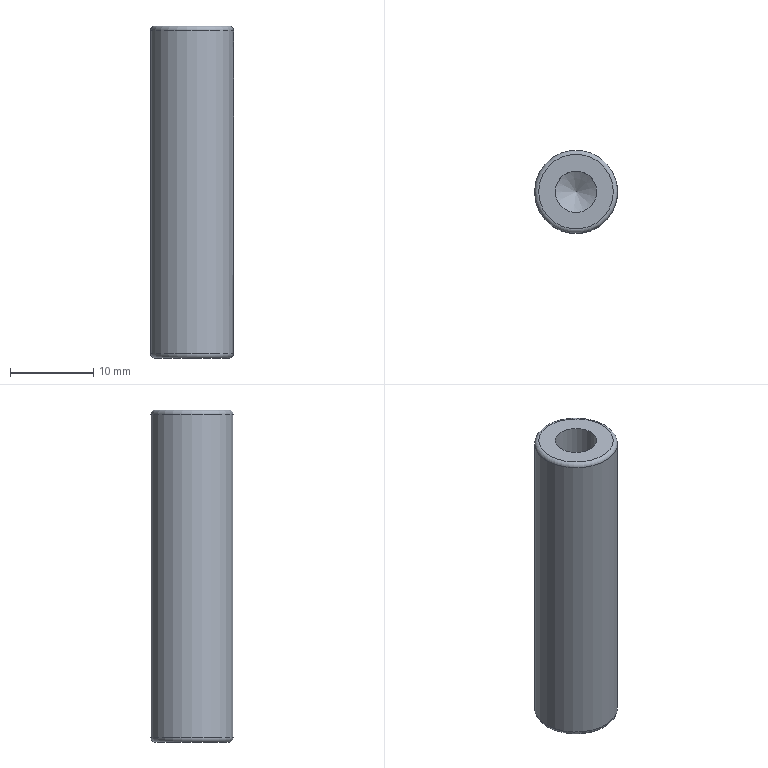Part | STEP file | solid 76 | 1 solid | 85 faces | box 10 x 10 x 40 mm | volume 2931 mm3 | plane 51 | other 24 | cylinder 7 | torus 2 | cone 1 | commonest cylinder face diameters 10 x6 5 x1